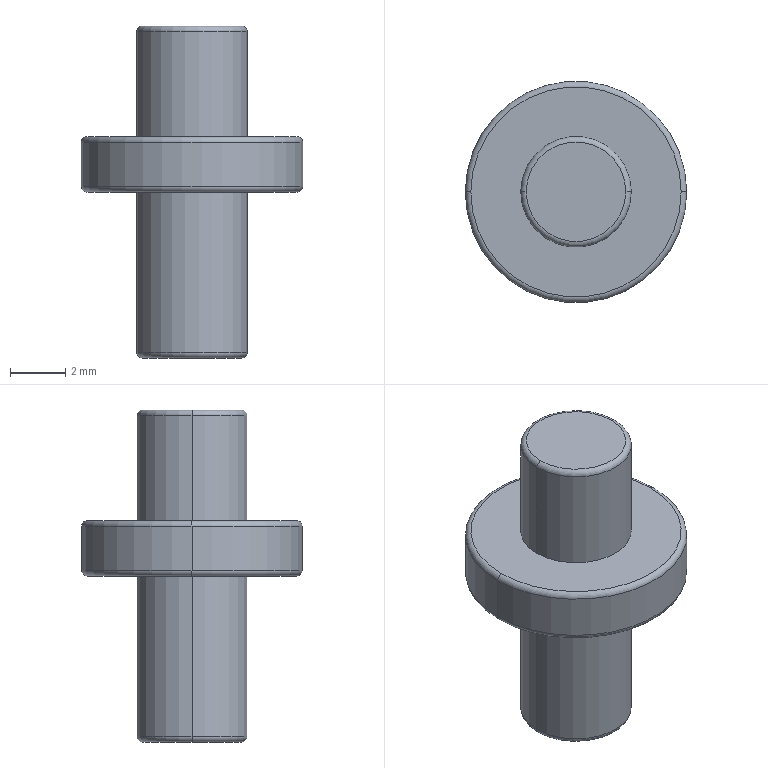Part | SolidWorks | features Fillet 2, ICE 2, Extrusion 1 | 1 solid | 18 faces | box 8 x 8 x 12 mm | volume 225.557 mm3 | torus 8 | cylinder 6 | plane 4 | commonest cylinder face diameters 4 x4 8 x2
STEP:
#1=CARTESIAN_POINT('',(-3.8,0.,6.));
#2=VERTEX_POINT('',#1);
#3=CARTESIAN_POINT('',(3.8,0.,6.));
#4=VERTEX_POINT('',#3);
#5=CARTESIAN_POINT('',(0.,0.,6.));
#6=DIRECTION('',(0.,0.,-1.));
#7=DIRECTION('',(1.,0.,0.));
#8=AXIS2_PLACEMENT_3D('',#5,#6,#7);
#9=CIRCLE('',#8,3.8);
#10=EDGE_CURVE('',#2,#4,#9,.T.);
#11=ORIENTED_EDGE('',*,*,#10,.F.);
#12=CARTESIAN_POINT('',(-4.,0.,6.2));
#13=VERTEX_POINT('',#12);
#14=CARTESIAN_POINT('',(-3.8,0.,6.2));
#15=DIRECTION('',(0.,1.,0.));
#16=DIRECTION('',(-1.,0.,0.));
#17=AXIS2_PLACEMENT_3D('',#14,#15,#16);
#18=CIRCLE('',#17,0.2);
#19=EDGE_CURVE('',#2,#13,#18,.T.);
#20=ORIENTED_EDGE('',*,*,#19,.T.);
#21=CARTESIAN_POINT('',(4.,0.,6.2));
#22=VERTEX_POINT('',#21);
#23=CARTESIAN_POINT('',(0.,0.,6.2));
#24=DIRECTION('',(0.,0.,1.));
#25=DIRECTION('',(1.,0.,0.));
#26=AXIS2_PLACEMENT_3D('',#23,#24,#25);
#27=CIRCLE('',#26,4.);
#28=EDGE_CURVE('',#22,#13,#27,.T.);
#29=ORIENTED_EDGE('',*,*,#28,.F.);
#30=CARTESIAN_POINT('',(3.8,0.,6.2));
#31=DIRECTION('',(0.,-1.,0.));
#32=DIRECTION('',(0.,0.,-1.));
#33=AXIS2_PLACEMENT_3D('',#30,#31,#32);
#34=CIRCLE('',#33,0.2);
#35=EDGE_CURVE('',#4,#22,#34,.T.);
#36=ORIENTED_EDGE('',*,*,#35,.F.);
#37=EDGE_LOOP('',(#11,#20,#29,#36));
#38=FACE_OUTER_BOUND('',#37,.T.);
#39=CARTESIAN_POINT('',(0.,0.,6.2));
#40=DIRECTION('',(0.,0.,1.));
#41=DIRECTION('',(1.,0.,0.));
#42=AXIS2_PLACEMENT_3D('',#39,#40,#41);
#43=TOROIDAL_SURFACE('',#42,3.8,0.2);
#44=ADVANCED_FACE('',(#38),#43,.T.);
#45=CARTESIAN_POINT('',(-4.,0.,7.8));
#46=VERTEX_POINT('',#45);
#47=CARTESIAN_POINT('',(4.,0.,7.8));
#48=VERTEX_POINT('',#47);
#49=CARTESIAN_POINT('',(0.,0.,7.8));
#50=DIRECTION('',(0.,0.,-1.));
#51=DIRECTION('',(1.,0.,0.));
#52=AXIS2_PLACEMENT_3D('',#49,#50,#51);
#53=CIRCLE('',#52,4.);
#54=EDGE_CURVE('',#46,#48,#53,.T.);
#55=ORIENTED_EDGE('',*,*,#54,.F.);
#56=CARTESIAN_POINT('',(-3.8,0.,8.));
#57=VERTEX_POINT('',#56);
#58=CARTESIAN_POINT('',(-3.8,0.,7.8));
#59=DIRECTION('',(0.,1.,0.));
#60=DIRECTION('',(-1.,0.,0.));
#61=AXIS2_PLACEMENT_3D('',#58,#59,#60);
#62=CIRCLE('',#61,0.2);
#63=EDGE_CURVE('',#46,#57,#62,.T.);
#64=ORIENTED_EDGE('',*,*,#63,.T.);
#65=CARTESIAN_POINT('',(3.8,0.,8.));
#66=VERTEX_POINT('',#65);
#67=CARTESIAN_POINT('',(0.,0.,8.));
#68=DIRECTION('',(0.,0.,1.));
#69=DIRECTION('',(1.,0.,0.));
#70=AXIS2_PLACEMENT_3D('',#67,#68,#69);
#71=CIRCLE('',#70,3.8);
#72=EDGE_CURVE('',#66,#57,#71,.T.);
#73=ORIENTED_EDGE('',*,*,#72,.F.);
#74=CARTESIAN_POINT('',(3.8,0.,7.8));
#75=DIRECTION('',(0.,-1.,0.));
#76=DIRECTION('',(0.,0.,-1.));
#77=AXIS2_PLACEMENT_3D('',#74,#75,#76);
#78=CIRCLE('',#77,0.2);
#79=EDGE_CURVE('',#48,#66,#78,.T.);
#80=ORIENTED_EDGE('',*,*,#79,.F.);
#81=EDGE_LOOP('',(#55,#64,#73,#80));
#82=FACE_OUTER_BOUND('',#81,.T.);
#83=CARTESIAN_POINT('',(0.,0.,7.8));
#84=DIRECTION('',(0.,0.,1.));
#85=DIRECTION('',(1.,0.,0.));
#86=AXIS2_PLACEMENT_3D('',#83,#84,#85);
#87=TOROIDAL_SURFACE('',#86,3.8,0.2);
#88=ADVANCED_FACE('',(#82),#87,.T.);
#89=CARTESIAN_POINT('',(-2.,0.,11.8));
#90=VERTEX_POINT('',#89);
#91=CARTESIAN_POINT('',(2.,0.,11.8));
#92=VERTEX_POINT('',#91);
#93=CARTESIAN_POINT('',(0.,0.,11.8));
#94=DIRECTION('',(0.,0.,-1.));
#95=DIRECTION('',(1.,0.,0.));
#96=AXIS2_PLACEMENT_3D('',#93,#94,#95);
#97=CIRCLE('',#96,2.);
#98=EDGE_CURVE('',#90,#92,#97,.T.);
#99=ORIENTED_EDGE('',*,*,#98,.F.);
#100=CARTESIAN_POINT('',(-1.8,0.,12.));
#101=VERTEX_POINT('',#100);
#102=CARTESIAN_POINT('',(-1.8,0.,11.8));
#103=DIRECTION('',(0.,1.,0.));
#104=DIRECTION('',(-1.,0.,0.));
#105=AXIS2_PLACEMENT_3D('',#102,#103,#104);
#106=CIRCLE('',#105,0.2);
#107=EDGE_CURVE('',#90,#101,#106,.T.);
#108=ORIENTED_EDGE('',*,*,#107,.T.);
#109=CARTESIAN_POINT('',(1.8,0.,12.));
#110=VERTEX_POINT('',#109);
#111=CARTESIAN_POINT('',(0.,0.,12.));
#112=DIRECTION('',(0.,0.,1.));
#113=DIRECTION('',(1.,0.,0.));
#114=AXIS2_PLACEMENT_3D('',#111,#112,#113);
#115=CIRCLE('',#114,1.8);
#116=EDGE_CURVE('',#110,#101,#115,.T.);
#117=ORIENTED_EDGE('',*,*,#116,.F.);
#118=CARTESIAN_POINT('',(1.8,0.,11.8));
#119=DIRECTION('',(0.,-1.,0.));
#120=DIRECTION('',(0.,0.,-1.));
#121=AXIS2_PLACEMENT_3D('',#118,#119,#120);
#122=CIRCLE('',#121,0.2);
#123=EDGE_CURVE('',#92,#110,#122,.T.);
#124=ORIENTED_EDGE('',*,*,#123,.F.);
#125=EDGE_LOOP('',(#99,#108,#117,#124));
#126=FACE_OUTER_BOUND('',#125,.T.);
#127=CARTESIAN_POINT('',(0.,0.,11.8));
#128=DIRECTION('',(0.,0.,1.));
#129=DIRECTION('',(1.,0.,0.));
#130=AXIS2_PLACEMENT_3D('',#127,#128,#129);
#131=TOROIDAL_SURFACE('',#130,1.8,0.2);
#132=ADVANCED_FACE('',(#126),#131,.T.);
#133=CARTESIAN_POINT('',(-1.8,0.,0.));
#134=VERTEX_POINT('',#133);
#135=CARTESIAN_POINT('',(1.8,0.,0.));
#136=VERTEX_POINT('',#135);
#137=CARTESIAN_POINT('',(0.,0.,0.));
#138=DIRECTION('',(0.,0.,-1.));
#139=DIRECTION('',(1.,0.,0.));
#140=AXIS2_PLACEMENT_3D('',#137,#138,#139);
#141=CIRCLE('',#140,1.8);
#142=EDGE_CURVE('',#134,#136,#141,.T.);
#143=ORIENTED_EDGE('',*,*,#142,.F.);
#144=CARTESIAN_POINT('',(-2.,0.,0.2));
#145=VERTEX_POINT('',#144);
#146=CARTESIAN_POINT('',(-1.8,0.,0.2));
#147=DIRECTION('',(0.,1.,0.));
#148=DIRECTION('',(-1.,0.,0.));
#149=AXIS2_PLACEMENT_3D('',#146,#147,#148);
#150=CIRCLE('',#149,0.2);
#151=EDGE_CURVE('',#134,#145,#150,.T.);
#152=ORIENTED_EDGE('',*,*,#151,.T.);
#153=CARTESIAN_POINT('',(2.,0.,0.2));
#154=VERTEX_POINT('',#153);
#155=CARTESIAN_POINT('',(0.,0.,0.2));
#156=DIRECTION('',(0.,0.,1.));
#157=DIRECTION('',(1.,0.,0.));
#158=AXIS2_PLACEMENT_3D('',#155,#156,#157);
#159=CIRCLE('',#158,2.);
#160=EDGE_CURVE('',#154,#145,#159,.T.);
#161=ORIENTED_EDGE('',*,*,#160,.F.);
#162=CARTESIAN_POINT('',(1.8,0.,0.2));
#163=DIRECTION('',(0.,-1.,0.));
#164=DIRECTION('',(0.,0.,-1.));
#165=AXIS2_PLACEMENT_3D('',#162,#163,#164);
#166=CIRCLE('',#165,0.2);
#167=EDGE_CURVE('',#136,#154,#166,.T.);
#168=ORIENTED_EDGE('',*,*,#167,.F.);
#169=EDGE_LOOP('',(#143,#152,#161,#168));
#170=FACE_OUTER_BOUND('',#169,.T.);
#171=CARTESIAN_POINT('',(0.,0.,0.2));
#172=DIRECTION('',(0.,0.,1.));
#173=DIRECTION('',(1.,0.,0.));
#174=AXIS2_PLACEMENT_3D('',#171,#172,#173);
#175=TOROIDAL_SURFACE('',#174,1.8,0.2);
#176=ADVANCED_FACE('',(#170),#175,.T.);
#177=ORIENTED_EDGE('',*,*,#98,.T.);
#178=CARTESIAN_POINT('',(2.,0.,8.));
#179=VERTEX_POINT('',#178);
#180=CARTESIAN_POINT('',(2.,0.,12.));
#181=DIRECTION('',(0.,0.,-1.));
#182=VECTOR('',#181,1000.);
#183=LINE('',#180,#182);
#184=EDGE_CURVE('',#92,#179,#183,.T.);
#185=ORIENTED_EDGE('',*,*,#184,.T.);
#186=CARTESIAN_POINT('',(-2.,0.,8.));
#187=VERTEX_POINT('',#186);
#188=CARTESIAN_POINT('',(0.,0.,8.));
#189=DIRECTION('',(0.,0.,1.));
#190=DIRECTION('',(1.,0.,0.));
#191=AXIS2_PLACEMENT_3D('',#188,#189,#190);
#192=CIRCLE('',#191,2.);
#193=EDGE_CURVE('',#179,#187,#192,.T.);
#194=ORIENTED_EDGE('',*,*,#193,.T.);
#195=CARTESIAN_POINT('',(-2.,0.,12.));
#196=DIRECTION('',(0.,0.,-1.));
#197=VECTOR('',#196,1000.);
#198=LINE('',#195,#197);
#199=EDGE_CURVE('',#90,#187,#198,.T.);
#200=ORIENTED_EDGE('',*,*,#199,.F.);
#201=EDGE_LOOP('',(#177,#185,#194,#200));
#202=FACE_OUTER_BOUND('',#201,.T.);
#203=CARTESIAN_POINT('',(0.,0.,12.));
#204=DIRECTION('',(0.,0.,-1.));
#205=DIRECTION('',(-1.,0.,0.));
#206=AXIS2_PLACEMENT_3D('',#203,#204,#205);
#207=CYLINDRICAL_SURFACE('',#206,2.);
#208=ADVANCED_FACE('',(#202),#207,.T.);
#209=ORIENTED_EDGE('',*,*,#54,.T.);
#210=CARTESIAN_POINT('',(4.,0.,8.));
#211=DIRECTION('',(0.,0.,-1.));
#212=VECTOR('',#211,1000.);
#213=LINE('',#210,#212);
#214=EDGE_CURVE('',#48,#22,#213,.T.);
#215=ORIENTED_EDGE('',*,*,#214,.T.);
#216=ORIENTED_EDGE('',*,*,#28,.T.);
#217=CARTESIAN_POINT('',(-4.,0.,8.));
#218=DIRECTION('',(0.,0.,-1.));
#219=VECTOR('',#218,1000.);
#220=LINE('',#217,#219);
#221=EDGE_CURVE('',#46,#13,#220,.T.);
#222=ORIENTED_EDGE('',*,*,#221,.F.);
#223=EDGE_LOOP('',(#209,#215,#216,#222));
#224=FACE_OUTER_BOUND('',#223,.T.);
#225=CARTESIAN_POINT('',(0.,0.,8.));
#226=DIRECTION('',(0.,0.,-1.));
#227=DIRECTION('',(-1.,0.,0.));
#228=AXIS2_PLACEMENT_3D('',#225,#226,#227);
#229=CYLINDRICAL_SURFACE('',#228,4.);
#230=ADVANCED_FACE('',(#224),#229,.T.);
#231=CARTESIAN_POINT('',(2.,0.,6.));
#232=VERTEX_POINT('',#231);
#233=CARTESIAN_POINT('',(-2.,0.,6.));
#234=VERTEX_POINT('',#233);
#235=CARTESIAN_POINT('',(0.,0.,6.));
#236=DIRECTION('',(0.,0.,1.));
#237=DIRECTION('',(1.,0.,0.));
#238=AXIS2_PLACEMENT_3D('',#235,#236,#237);
#239=CIRCLE('',#238,2.);
#240=EDGE_CURVE('',#232,#234,#239,.T.);
#241=ORIENTED_EDGE('',*,*,#240,.F.);
#242=CARTESIAN_POINT('',(2.,0.,6.));
#243=DIRECTION('',(0.,0.,-1.));
#244=VECTOR('',#243,1000.);
#245=LINE('',#242,#244);
#246=EDGE_CURVE('',#232,#154,#245,.T.);
#247=ORIENTED_EDGE('',*,*,#246,.T.);
#248=ORIENTED_EDGE('',*,*,#160,.T.);
#249=CARTESIAN_POINT('',(-2.,0.,6.));
#250=DIRECTION('',(0.,0.,-1.));
#251=VECTOR('',#250,1000.);
#252=LINE('',#249,#251);
#253=EDGE_CURVE('',#234,#145,#252,.T.);
#254=ORIENTED_EDGE('',*,*,#253,.F.);
#255=EDGE_LOOP('',(#241,#247,#248,#254));
#256=FACE_OUTER_BOUND('',#255,.T.);
#257=CARTESIAN_POINT('',(0.,0.,6.));
#258=DIRECTION('',(0.,0.,-1.));
#259=DIRECTION('',(-1.,0.,0.));
#260=AXIS2_PLACEMENT_3D('',#257,#258,#259);
#261=CYLINDRICAL_SURFACE('',#260,2.);
#262=ADVANCED_FACE('',(#256),#261,.T.);
#263=ORIENTED_EDGE('',*,*,#72,.T.);
#264=CARTESIAN_POINT('',(0.,0.,8.));
#265=DIRECTION('',(0.,0.,1.));
#266=DIRECTION('',(1.,0.,0.));
#267=AXIS2_PLACEMENT_3D('',#264,#265,#266);
#268=CIRCLE('',#267,3.8);
#269=EDGE_CURVE('',#57,#66,#268,.T.);
#270=ORIENTED_EDGE('',*,*,#269,.T.);
#271=EDGE_LOOP('',(#263,#270));
#272=FACE_OUTER_BOUND('',#271,.T.);
#273=CARTESIAN_POINT('',(0.,0.,8.));
#274=DIRECTION('',(0.,0.,1.));
#275=DIRECTION('',(1.,0.,0.));
#276=AXIS2_PLACEMENT_3D('',#273,#274,#275);
#277=CIRCLE('',#276,2.);
#278=EDGE_CURVE('',#187,#179,#277,.T.);
#279=ORIENTED_EDGE('',*,*,#278,.F.);
#280=ORIENTED_EDGE('',*,*,#193,.F.);
#281=EDGE_LOOP('',(#279,#280));
#282=FACE_BOUND('',#281,.T.);
#283=CARTESIAN_POINT('',(0.,0.,8.));
#284=DIRECTION('',(0.,0.,1.));
#285=DIRECTION('',(1.,0.,0.));
#286=AXIS2_PLACEMENT_3D('',#283,#284,#285);
#287=PLANE('',#286);
#288=ADVANCED_FACE('',(#272,#282),#287,.T.);
#289=ORIENTED_EDGE('',*,*,#246,.F.);
#290=CARTESIAN_POINT('',(0.,0.,6.));
#291=DIRECTION('',(0.,0.,1.));
#292=DIRECTION('',(1.,0.,0.));
#293=AXIS2_PLACEMENT_3D('',#290,#291,#292);
#294=CIRCLE('',#293,2.);
#295=EDGE_CURVE('',#234,#232,#294,.T.);
#296=ORIENTED_EDGE('',*,*,#295,.F.);
#297=ORIENTED_EDGE('',*,*,#253,.T.);
#298=CARTESIAN_POINT('',(0.,0.,0.2));
#299=DIRECTION('',(0.,0.,1.));
#300=DIRECTION('',(1.,0.,0.));
#301=AXIS2_PLACEMENT_3D('',#298,#299,#300);
#302=CIRCLE('',#301,2.);
#303=EDGE_CURVE('',#145,#154,#302,.T.);
#304=ORIENTED_EDGE('',*,*,#303,.T.);
#305=EDGE_LOOP('',(#289,#296,#297,#304));
#306=FACE_OUTER_BOUND('',#305,.T.);
#307=CARTESIAN_POINT('',(0.,0.,6.));
#308=DIRECTION('',(0.,0.,-1.));
#309=DIRECTION('',(-1.,0.,0.));
#310=AXIS2_PLACEMENT_3D('',#307,#308,#309);
#311=CYLINDRICAL_SURFACE('',#310,2.);
#312=ADVANCED_FACE('',(#306),#311,.T.);
#313=CARTESIAN_POINT('',(0.,0.,0.));
#314=DIRECTION('',(0.,0.,-1.));
#315=DIRECTION('',(1.,0.,0.));
#316=AXIS2_PLACEMENT_3D('',#313,#314,#315);
#317=CIRCLE('',#316,1.8);
#318=EDGE_CURVE('',#136,#134,#317,.T.);
#319=ORIENTED_EDGE('',*,*,#318,.T.);
#320=ORIENTED_EDGE('',*,*,#142,.T.);
#321=EDGE_LOOP('',(#319,#320));
#322=FACE_OUTER_BOUND('',#321,.T.);
#323=CARTESIAN_POINT('',(0.,0.,0.));
#324=DIRECTION('',(0.,0.,1.));
#325=DIRECTION('',(1.,0.,0.));
#326=AXIS2_PLACEMENT_3D('',#323,#324,#325);
#327=PLANE('',#326);
#328=ADVANCED_FACE('',(#322),#327,.F.);
#329=CARTESIAN_POINT('',(0.,0.,6.));
#330=DIRECTION('',(0.,0.,-1.));
#331=DIRECTION('',(1.,0.,0.));
#332=AXIS2_PLACEMENT_3D('',#329,#330,#331);
#333=CIRCLE('',#332,3.8);
#334=EDGE_CURVE('',#4,#2,#333,.T.);
#335=ORIENTED_EDGE('',*,*,#334,.T.);
#336=ORIENTED_EDGE('',*,*,#10,.T.);
#337=EDGE_LOOP('',(#335,#336));
#338=FACE_OUTER_BOUND('',#337,.T.);
#339=ORIENTED_EDGE('',*,*,#295,.T.);
#340=ORIENTED_EDGE('',*,*,#240,.T.);
#341=EDGE_LOOP('',(#339,#340));
#342=FACE_BOUND('',#341,.T.);
#343=CARTESIAN_POINT('',(0.,0.,6.));
#344=DIRECTION('',(0.,0.,1.));
#345=DIRECTION('',(1.,0.,0.));
#346=AXIS2_PLACEMENT_3D('',#343,#344,#345);
#347=PLANE('',#346);
#348=ADVANCED_FACE('',(#338,#342),#347,.F.);
#349=ORIENTED_EDGE('',*,*,#214,.F.);
#350=CARTESIAN_POINT('',(0.,0.,7.8));
#351=DIRECTION('',(0.,0.,-1.));
#352=DIRECTION('',(1.,0.,0.));
#353=AXIS2_PLACEMENT_3D('',#350,#351,#352);
#354=CIRCLE('',#353,4.);
#355=EDGE_CURVE('',#48,#46,#354,.T.);
#356=ORIENTED_EDGE('',*,*,#355,.T.);
#357=ORIENTED_EDGE('',*,*,#221,.T.);
#358=CARTESIAN_POINT('',(0.,0.,6.2));
#359=DIRECTION('',(0.,0.,1.));
#360=DIRECTION('',(1.,0.,0.));
#361=AXIS2_PLACEMENT_3D('',#358,#359,#360);
#362=CIRCLE('',#361,4.);
#363=EDGE_CURVE('',#13,#22,#362,.T.);
#364=ORIENTED_EDGE('',*,*,#363,.T.);
#365=EDGE_LOOP('',(#349,#356,#357,#364));
#366=FACE_OUTER_BOUND('',#365,.T.);
#367=CARTESIAN_POINT('',(0.,0.,8.));
#368=DIRECTION('',(0.,0.,-1.));
#369=DIRECTION('',(-1.,0.,0.));
#370=AXIS2_PLACEMENT_3D('',#367,#368,#369);
#371=CYLINDRICAL_SURFACE('',#370,4.);
#372=ADVANCED_FACE('',(#366),#371,.T.);
#373=ORIENTED_EDGE('',*,*,#184,.F.);
#374=CARTESIAN_POINT('',(0.,0.,11.8));
#375=DIRECTION('',(0.,0.,-1.));
#376=DIRECTION('',(1.,0.,0.));
#377=AXIS2_PLACEMENT_3D('',#374,#375,#376);
#378=CIRCLE('',#377,2.);
#379=EDGE_CURVE('',#92,#90,#378,.T.);
#380=ORIENTED_EDGE('',*,*,#379,.T.);
#381=ORIENTED_EDGE('',*,*,#199,.T.);
#382=ORIENTED_EDGE('',*,*,#278,.T.);
#383=EDGE_LOOP('',(#373,#380,#381,#382));
#384=FACE_OUTER_BOUND('',#383,.T.);
#385=CARTESIAN_POINT('',(0.,0.,12.));
#386=DIRECTION('',(0.,0.,-1.));
#387=DIRECTION('',(-1.,0.,0.));
#388=AXIS2_PLACEMENT_3D('',#385,#386,#387);
#389=CYLINDRICAL_SURFACE('',#388,2.);
#390=ADVANCED_FACE('',(#384),#389,.T.);
#391=ORIENTED_EDGE('',*,*,#116,.T.);
#392=CARTESIAN_POINT('',(0.,0.,12.));
#393=DIRECTION('',(0.,0.,1.));
#394=DIRECTION('',(1.,0.,0.));
#395=AXIS2_PLACEMENT_3D('',#392,#393,#394);
#396=CIRCLE('',#395,1.8);
#397=EDGE_CURVE('',#101,#110,#396,.T.);
#398=ORIENTED_EDGE('',*,*,#397,.T.);
#399=EDGE_LOOP('',(#391,#398));
#400=FACE_OUTER_BOUND('',#399,.T.);
#401=CARTESIAN_POINT('',(0.,0.,12.));
#402=DIRECTION('',(0.,0.,1.));
#403=DIRECTION('',(1.,0.,0.));
#404=AXIS2_PLACEMENT_3D('',#401,#402,#403);
#405=PLANE('',#404);
#406=ADVANCED_FACE('',(#400),#405,.T.);
#407=ORIENTED_EDGE('',*,*,#151,.F.);
#408=ORIENTED_EDGE('',*,*,#318,.F.);
#409=ORIENTED_EDGE('',*,*,#167,.T.);
#410=ORIENTED_EDGE('',*,*,#303,.F.);
#411=EDGE_LOOP('',(#407,#408,#409,#410));
#412=FACE_OUTER_BOUND('',#411,.T.);
#413=CARTESIAN_POINT('',(0.,0.,0.2));
#414=DIRECTION('',(0.,0.,1.));
#415=DIRECTION('',(1.,0.,0.));
#416=AXIS2_PLACEMENT_3D('',#413,#414,#415);
#417=TOROIDAL_SURFACE('',#416,1.8,0.2);
#418=ADVANCED_FACE('',(#412),#417,.T.);
#419=ORIENTED_EDGE('',*,*,#107,.F.);
#420=ORIENTED_EDGE('',*,*,#379,.F.);
#421=ORIENTED_EDGE('',*,*,#123,.T.);
#422=ORIENTED_EDGE('',*,*,#397,.F.);
#423=EDGE_LOOP('',(#419,#420,#421,#422));
#424=FACE_OUTER_BOUND('',#423,.T.);
#425=CARTESIAN_POINT('',(0.,0.,11.8));
#426=DIRECTION('',(0.,0.,1.));
#427=DIRECTION('',(1.,0.,0.));
#428=AXIS2_PLACEMENT_3D('',#425,#426,#427);
#429=TOROIDAL_SURFACE('',#428,1.8,0.2);
#430=ADVANCED_FACE('',(#424),#429,.T.);
#431=ORIENTED_EDGE('',*,*,#63,.F.);
#432=ORIENTED_EDGE('',*,*,#355,.F.);
#433=ORIENTED_EDGE('',*,*,#79,.T.);
#434=ORIENTED_EDGE('',*,*,#269,.F.);
#435=EDGE_LOOP('',(#431,#432,#433,#434));
#436=FACE_OUTER_BOUND('',#435,.T.);
#437=CARTESIAN_POINT('',(0.,0.,7.8));
#438=DIRECTION('',(0.,0.,1.));
#439=DIRECTION('',(1.,0.,0.));
#440=AXIS2_PLACEMENT_3D('',#437,#438,#439);
#441=TOROIDAL_SURFACE('',#440,3.8,0.2);
#442=ADVANCED_FACE('',(#436),#441,.T.);
#443=ORIENTED_EDGE('',*,*,#19,.F.);
#444=ORIENTED_EDGE('',*,*,#334,.F.);
#445=ORIENTED_EDGE('',*,*,#35,.T.);
#446=ORIENTED_EDGE('',*,*,#363,.F.);
#447=EDGE_LOOP('',(#443,#444,#445,#446));
#448=FACE_OUTER_BOUND('',#447,.T.);
#449=CARTESIAN_POINT('',(0.,0.,6.2));
#450=DIRECTION('',(0.,0.,1.));
#451=DIRECTION('',(1.,0.,0.));
#452=AXIS2_PLACEMENT_3D('',#449,#450,#451);
#453=TOROIDAL_SURFACE('',#452,3.8,0.2);
#454=ADVANCED_FACE('',(#448),#453,.T.);
#455=CLOSED_SHELL('',(#44,#88,#132,#176,#208,#230,#262,#288,#312,#328,#348,#372,#390,#406,#418,#430,#442,#454));
#456=MANIFOLD_SOLID_BREP('',#455);
#457=CARTESIAN_POINT('',(0.,0.,0.));
#458=DIRECTION('',(0.,0.,1.));
#459=DIRECTION('',(1.,0.,0.));
#460=AXIS2_PLACEMENT_3D('',#457,#458,#459);
#461=(LENGTH_UNIT()NAMED_UNIT(*)SI_UNIT(.MILLI.,.METRE.));
#462=UNCERTAINTY_MEASURE_WITH_UNIT(LENGTH_MEASURE(0.00001),#461,'','');
#463=(NAMED_UNIT(*)PLANE_ANGLE_UNIT()SI_UNIT($,.RADIAN.));
#464=(NAMED_UNIT(*)SI_UNIT($,.STERADIAN.)SOLID_ANGLE_UNIT());
#465=(GEOMETRIC_REPRESENTATION_CONTEXT(3)GLOBAL_UNCERTAINTY_ASSIGNED_CONTEXT((#462))GLOBAL_UNIT_ASSIGNED_CONTEXT((#461,#463,#464))REPRESENTATION_CONTEXT('',''));
#466=ADVANCED_BREP_SHAPE_REPRESENTATION('',(#456,#460),#465);